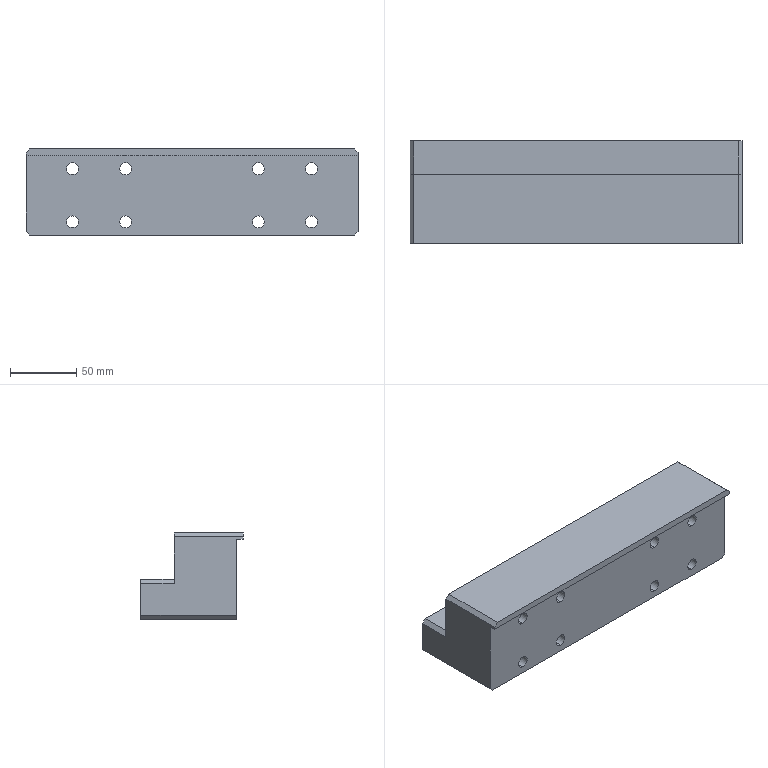Part | SolidWorks | features HoleWzd 6, ICE 2, Chamfer 1, Extrusion 1, MirrorPattern 1 | 1 solid | 100 faces | box 250 x 77 x 65 mm | volume 889815 mm3 | cylinder 54 | plane 24 | cone 22 | commonest cylinder face diameters 6.8 x16 9 x16 15 x16 3.3 x4 8 x2